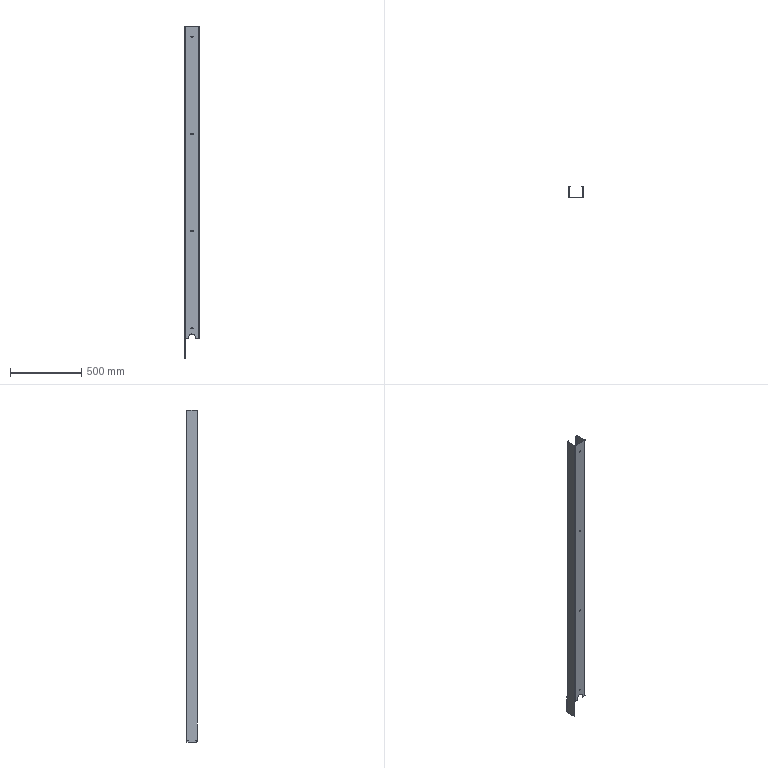Part | SolidWorks | features ICE 5, Fillet 2, LPattern 2, SMBaseFlange 2, Chamfer 1, FlatPattern 1, SheetMetal 1 | 1 solid | 99 faces | box 100 x 80 x 2323 mm | volume 934752 mm3 | cylinder 48 | plane 47 | cone 4 | commonest cylinder face diameters 6.4 x24 6 x12 2 x4 5 x4 10 x2 50 x2